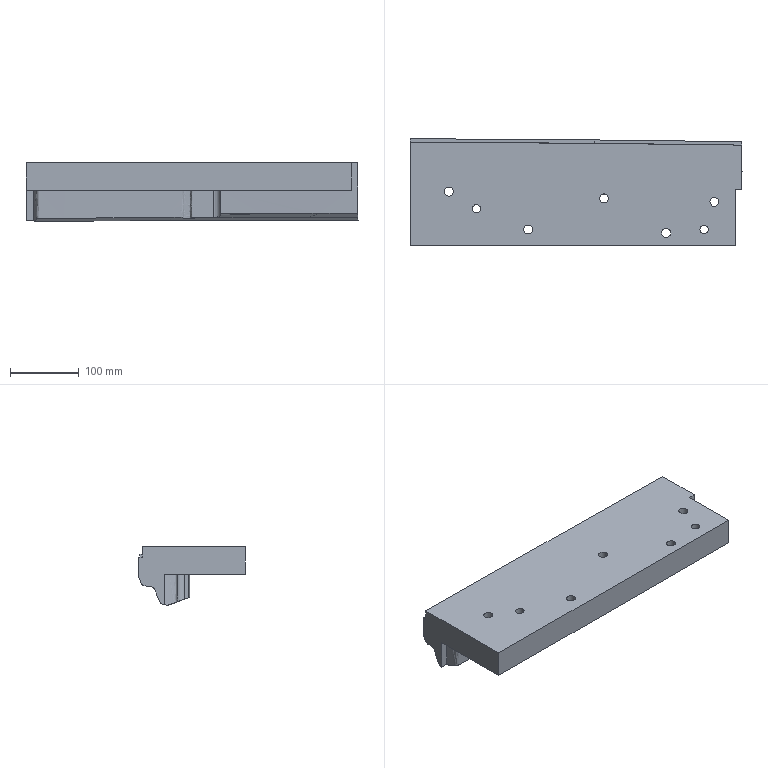Part | NX | features solid 2 | 1 solid | 87 faces | box 481.224 x 154.383 x 84.97 mm | volume 3683495 mm3 | spline 54 | plane 18 | cylinder 15 | commonest cylinder face diameters 13 x7 20 x6 12 x2